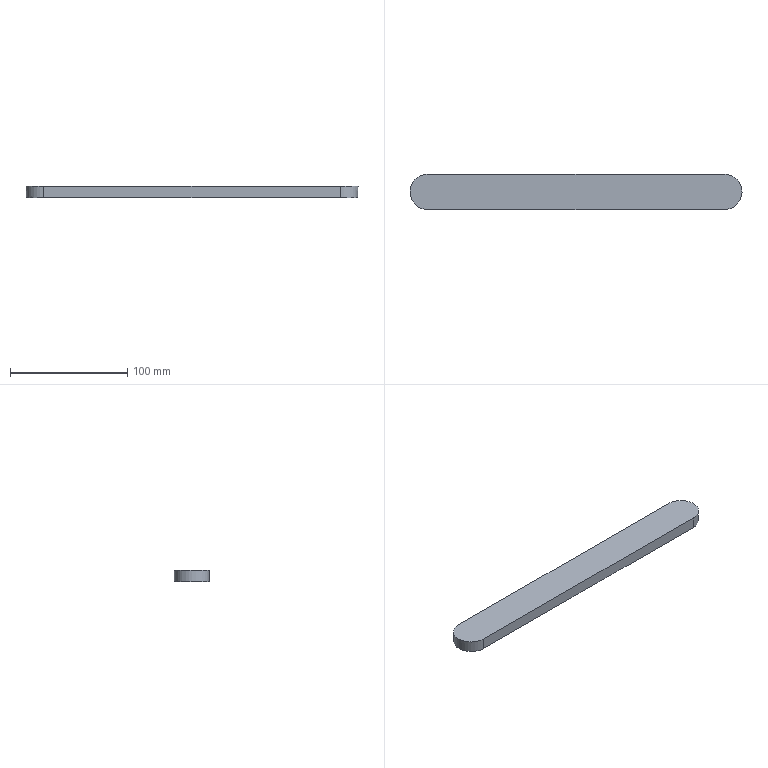Part | NX | features solid 2 | 1 solid | 6 faces | box 283.219 x 30 x 10 mm | volume 82945 mm3 | plane 4 | cylinder 2 | commonest cylinder face diameters 30 x2
STEP:
#1=CARTESIAN_POINT('',(126.603,-647.5,-10.));
#2=VERTEX_POINT('',#1);
#3=CARTESIAN_POINT('',(-126.603,-647.5,-10.));
#4=VERTEX_POINT('',#3);
#5=CARTESIAN_POINT('',(-10.,-647.5,-10.));
#6=DIRECTION('',(-1.,0.,0.));
#7=VECTOR('',#6,1000.);
#8=LINE('',#5,#7);
#9=EDGE_CURVE('',#2,#4,#8,.T.);
#10=ORIENTED_EDGE('',*,*,#9,.T.);
#11=CARTESIAN_POINT('',(-126.309,-647.5,-20.));
#12=VERTEX_POINT('',#11);
#13=CARTESIAN_POINT('',(-126.322,-647.5,-19.56));
#14=DIRECTION('',(-0.02934,0.,0.9996));
#15=VECTOR('',#14,1000.);
#16=LINE('',#13,#15);
#17=EDGE_CURVE('',#4,#12,#16,.F.);
#18=ORIENTED_EDGE('',*,*,#17,.T.);
#19=CARTESIAN_POINT('',(126.309,-647.5,-20.));
#20=VERTEX_POINT('',#19);
#21=CARTESIAN_POINT('',(-10.,-647.5,-20.));
#22=DIRECTION('',(-1.,0.,0.));
#23=VECTOR('',#22,1000.);
#24=LINE('',#21,#23);
#25=EDGE_CURVE('',#20,#12,#24,.T.);
#26=ORIENTED_EDGE('',*,*,#25,.F.);
#27=CARTESIAN_POINT('',(126.322,-647.5,-19.56));
#28=DIRECTION('',(0.02934,0.,0.9996));
#29=VECTOR('',#28,1000.);
#30=LINE('',#27,#29);
#31=EDGE_CURVE('',#2,#20,#30,.F.);
#32=ORIENTED_EDGE('',*,*,#31,.F.);
#33=EDGE_LOOP('',(#10,#18,#26,#32));
#34=FACE_BOUND('',#33,.T.);
#35=CARTESIAN_POINT('',(130.,-647.5,-10.));
#36=DIRECTION('',(0.,-1.,0.));
#37=DIRECTION('',(0.,0.,1.));
#38=AXIS2_PLACEMENT_3D('',#35,#36,#37);
#39=PLANE('',#38);
#40=ADVANCED_FACE('',(#34),#39,.T.);
#41=CARTESIAN_POINT('',(-126.309,-617.5,-20.));
#42=VERTEX_POINT('',#41);
#43=CARTESIAN_POINT('',(126.309,-617.5,-20.));
#44=VERTEX_POINT('',#43);
#45=CARTESIAN_POINT('',(-10.,-617.5,-20.));
#46=DIRECTION('',(1.,0.,0.));
#47=VECTOR('',#46,1000.);
#48=LINE('',#45,#47);
#49=EDGE_CURVE('',#42,#44,#48,.T.);
#50=ORIENTED_EDGE('',*,*,#49,.F.);
#51=CARTESIAN_POINT('',(-126.603,-617.5,-10.));
#52=VERTEX_POINT('',#51);
#53=CARTESIAN_POINT('',(-126.616,-617.5,-9.56));
#54=DIRECTION('',(0.02934,0.,-0.9996));
#55=VECTOR('',#54,1000.);
#56=LINE('',#53,#55);
#57=EDGE_CURVE('',#42,#52,#56,.F.);
#58=ORIENTED_EDGE('',*,*,#57,.T.);
#59=CARTESIAN_POINT('',(126.603,-617.5,-10.));
#60=VERTEX_POINT('',#59);
#61=CARTESIAN_POINT('',(-10.,-617.5,-10.));
#62=DIRECTION('',(1.,0.,0.));
#63=VECTOR('',#62,1000.);
#64=LINE('',#61,#63);
#65=EDGE_CURVE('',#52,#60,#64,.T.);
#66=ORIENTED_EDGE('',*,*,#65,.T.);
#67=CARTESIAN_POINT('',(126.616,-617.5,-9.56));
#68=DIRECTION('',(-0.02934,0.,-0.9996));
#69=VECTOR('',#68,1000.);
#70=LINE('',#67,#69);
#71=EDGE_CURVE('',#44,#60,#70,.F.);
#72=ORIENTED_EDGE('',*,*,#71,.F.);
#73=EDGE_LOOP('',(#50,#58,#66,#72));
#74=FACE_BOUND('',#73,.T.);
#75=CARTESIAN_POINT('',(-10.,-617.5,-10.));
#76=DIRECTION('',(0.,1.,0.));
#77=DIRECTION('',(0.,0.,-1.));
#78=AXIS2_PLACEMENT_3D('',#75,#76,#77);
#79=PLANE('',#78);
#80=ADVANCED_FACE('',(#74),#79,.T.);
#81=CARTESIAN_POINT('',(126.603,-632.5,-10.));
#82=DIRECTION('',(0.,0.,1.));
#83=DIRECTION('',(1.,0.,0.));
#84=AXIS2_PLACEMENT_3D('',#81,#82,#83);
#85=ELLIPSE('',#84,15.006,15.);
#86=EDGE_CURVE('',#60,#2,#85,.F.);
#87=ORIENTED_EDGE('',*,*,#86,.F.);
#88=ORIENTED_EDGE('',*,*,#65,.F.);
#89=CARTESIAN_POINT('',(-126.603,-632.5,-10.));
#90=DIRECTION('',(0.,0.,-1.));
#91=DIRECTION('',(-1.,0.,0.));
#92=AXIS2_PLACEMENT_3D('',#89,#90,#91);
#93=ELLIPSE('',#92,15.006,15.);
#94=EDGE_CURVE('',#52,#4,#93,.F.);
#95=ORIENTED_EDGE('',*,*,#94,.T.);
#96=ORIENTED_EDGE('',*,*,#9,.F.);
#97=EDGE_LOOP('',(#87,#88,#95,#96));
#98=FACE_BOUND('',#97,.T.);
#99=CARTESIAN_POINT('',(-10.,-650.,-10.));
#100=DIRECTION('',(0.,0.,-1.));
#101=DIRECTION('',(1.,0.,0.));
#102=AXIS2_PLACEMENT_3D('',#99,#100,#101);
#103=PLANE('',#102);
#104=ADVANCED_FACE('',(#98),#103,.F.);
#105=ORIENTED_EDGE('',*,*,#25,.T.);
#106=CARTESIAN_POINT('',(-126.309,-632.5,-20.));
#107=DIRECTION('',(0.,0.,-1.));
#108=DIRECTION('',(-1.,0.,0.));
#109=AXIS2_PLACEMENT_3D('',#106,#107,#108);
#110=ELLIPSE('',#109,15.006,15.);
#111=EDGE_CURVE('',#12,#42,#110,.T.);
#112=ORIENTED_EDGE('',*,*,#111,.T.);
#113=ORIENTED_EDGE('',*,*,#49,.T.);
#114=CARTESIAN_POINT('',(126.309,-632.5,-20.));
#115=DIRECTION('',(0.,0.,1.));
#116=DIRECTION('',(1.,0.,0.));
#117=AXIS2_PLACEMENT_3D('',#114,#115,#116);
#118=ELLIPSE('',#117,15.006,15.);
#119=EDGE_CURVE('',#20,#44,#118,.T.);
#120=ORIENTED_EDGE('',*,*,#119,.F.);
#121=EDGE_LOOP('',(#105,#112,#113,#120));
#122=FACE_BOUND('',#121,.T.);
#123=CARTESIAN_POINT('',(-10.,-650.,-20.));
#124=DIRECTION('',(0.,0.,-1.));
#125=DIRECTION('',(1.,0.,0.));
#126=AXIS2_PLACEMENT_3D('',#123,#124,#125);
#127=PLANE('',#126);
#128=ADVANCED_FACE('',(#122),#127,.T.);
#129=ORIENTED_EDGE('',*,*,#71,.T.);
#130=ORIENTED_EDGE('',*,*,#86,.T.);
#131=ORIENTED_EDGE('',*,*,#31,.T.);
#132=ORIENTED_EDGE('',*,*,#119,.T.);
#133=EDGE_LOOP('',(#129,#130,#131,#132));
#134=FACE_BOUND('',#133,.T.);
#135=CARTESIAN_POINT('',(127.498,-632.5,20.492));
#136=DIRECTION('',(0.02934,0.,0.9996));
#137=DIRECTION('',(-0.9996,0.,0.02934));
#138=AXIS2_PLACEMENT_3D('',#135,#136,#137);
#139=CYLINDRICAL_SURFACE('',#138,15.);
#140=ADVANCED_FACE('',(#134),#139,.T.);
#141=ORIENTED_EDGE('',*,*,#57,.F.);
#142=ORIENTED_EDGE('',*,*,#111,.F.);
#143=ORIENTED_EDGE('',*,*,#17,.F.);
#144=ORIENTED_EDGE('',*,*,#94,.F.);
#145=EDGE_LOOP('',(#141,#142,#143,#144));
#146=FACE_BOUND('',#145,.T.);
#147=CARTESIAN_POINT('',(-127.498,-632.5,20.492));
#148=DIRECTION('',(-0.02934,0.,0.9996));
#149=DIRECTION('',(0.9996,0.,0.02934));
#150=AXIS2_PLACEMENT_3D('',#147,#148,#149);
#151=CYLINDRICAL_SURFACE('',#150,15.);
#152=ADVANCED_FACE('',(#146),#151,.T.);
#153=CLOSED_SHELL('',(#40,#80,#104,#128,#140,#152));
#154=MANIFOLD_SOLID_BREP('',#153);
#155=(LENGTH_UNIT()NAMED_UNIT(*)SI_UNIT(.MILLI.,.METRE.));
#156=UNCERTAINTY_MEASURE_WITH_UNIT(LENGTH_MEASURE(0.00001),#155,'','');
#157=(NAMED_UNIT(*)PLANE_ANGLE_UNIT()SI_UNIT($,.RADIAN.));
#158=(NAMED_UNIT(*)SI_UNIT($,.STERADIAN.)SOLID_ANGLE_UNIT());
#159=(GEOMETRIC_REPRESENTATION_CONTEXT(3)GLOBAL_UNCERTAINTY_ASSIGNED_CONTEXT((#156))GLOBAL_UNIT_ASSIGNED_CONTEXT((#155,#157,#158))REPRESENTATION_CONTEXT('',''));
#160=ADVANCED_BREP_SHAPE_REPRESENTATION('',(#154),#159);